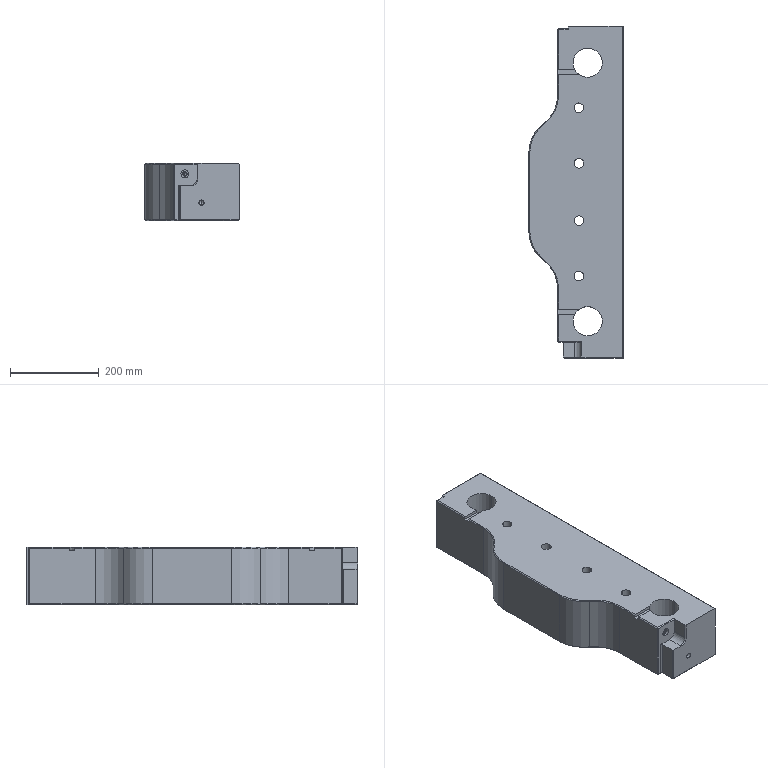Part | Creo | 1 solid | 294 faces | box 213 x 750 x 130 mm | volume 15735438 mm3 | plane 140 | other 68 | cylinder 56 | cone 30 | commonest cylinder face diameters 22 x8 6 x7 5 x6 14 x4 16 x4 66 x4